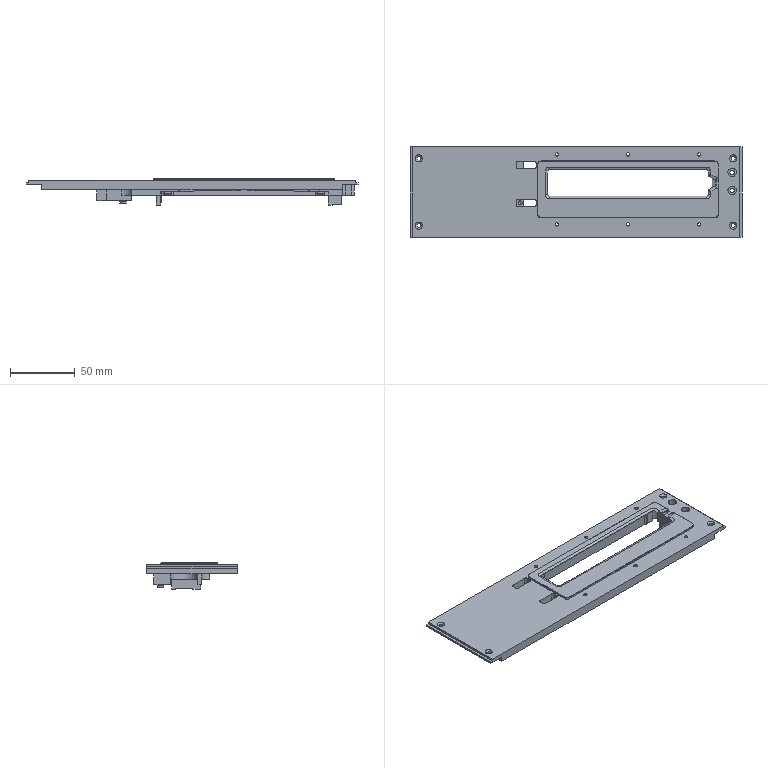NC program | NX | posted with a generic post | part box 256.6 x 70.3 x 20.422 mm
Lines 23 to 1070 of 15201:
(ADAPTIVE_MILLING , TOOL : D10)
N44 T10 M6
N46 G54
N48 G17 G0 G90 X-140.009 Y0.038 S9500 M3
N50 G43 Z30. H10
N52 Z-17.422
N54 G94 G1 Z-20.422 F1000.
N56 X-139.228 Y-0.241 F3000.
N58 X-138.44 Y-0.497
N60 G3 X-137.362 Y0.038 R1.017
N62 X-136.601 Y3.102 R8.28
N64 X-136.319 Y12.969 R111.643
N66 G1 X-136.314 Y15.219
N68 X-136.311 Y19.094
N70 X-136.31 Y32.719
N72 Y36.094
N74 X-136.305 Y36.344
N76 X-136.296 Y36.469
N78 G2 X-133.53 Y40.732 R5.992
N80 X-127.787 Y42.697 R13.242
N82 X-118.803 Y43.116 R74.905
N84 G1 X-117.428 Y43.124
N86 X-115.678 Y43.13
N88 X-113.178 Y43.135
N90 X-108.678 Y43.137
N92 X-67.178 Y43.138
N94 X129.322
N96 G2 X133.647 Y40.731 R5.631
N98 X135.753 Y35.309 R12.113
N100 X136.254 Y27.082 R56.828
N102 G1 X136.263 Y26.082
N104 X136.272 Y24.832
N106 X136.279 Y23.207
N108 X136.284 Y21.082
N110 X136.287 Y17.457
N112 X136.288 Y6.457
N114 Y-36.168
N116 X136.287 Y-36.293
N118 X136.281 Y-36.417
N120 X136.271 Y-36.542
N122 G2 X133.571 Y-40.712 R5.953
N124 X128.205 Y-42.64 R12.812
N126 X120.225 Y-43.103 R59.248
N128 G1 X119.225 Y-43.113
N130 X117.975 Y-43.122
N132 X116.35 Y-43.129
N134 X114.1 Y-43.134
N136 X110.35 Y-43.137
N138 X98.35 Y-43.138
N140 X1.1
N142 X0.475 Y-43.141
N144 X-1.275 Y-43.144
N146 X-2.9
N148 X-3.4 Y-43.143
N150 X-4.025 Y-43.145
N152 X-5.4 Y-43.146
N154 X-6.275 Y-43.145
N156 X-7.025 Y-43.147
N158 X-7.9
N160 X-8.525 Y-43.146
N162 X-9.65 Y-43.149
N164 X-10.525 Y-43.147
N166 X-11.65 Y-43.149
N168 X-12.65 Y-43.147
N170 X-13.525 Y-43.149
N172 X-15.025 Y-43.147
N174 X-15.775 Y-43.148
N176 X-16.775 Y-43.147
N178 X-17.4 Y-43.148
N180 X-18.275 Y-43.15
N182 X-19.15 Y-43.148
N184 X-20.4 Y-43.15
N186 X-21.65 Y-43.147
N188 X-22.275 Y-43.149
N190 X-23.775 Y-43.147
N192 X-24.525 Y-43.146
N194 X-25.275 Y-43.148
N196 X-26.15 Y-43.147
N198 X-26.525
N200 X-27.775 Y-43.15
N202 X-28.525 Y-43.148
N204 X-29.775 Y-43.15
N206 X-31.025 Y-43.147
N208 X-31.65 Y-43.148
N210 X-33.025 Y-43.147
N212 X-33.774 Y-43.146
N214 X-34.399 Y-43.147
N216 X-35.774
N218 X-36.524 Y-43.146
N220 X-37.399 Y-43.148
N222 X-38.524 Y-43.147
N224 X-39.399 Y-43.149
N226 X-40.399 Y-43.147
N228 X-40.899 Y-43.146
N230 X-41.649 Y-43.148
N232 X-42.649 Y-43.147
N234 X-43.274 Y-43.148
N236 X-44.149 Y-43.15
N238 X-45.024 Y-43.148
N240 X-46.149 Y-43.15
N242 X-46.899 Y-43.149
N244 X-48.149 Y-43.15
N246 X-49.524 Y-43.147
N248 X-50.899 Y-43.15
N250 X-52.024 Y-43.148
N252 X-52.774 Y-43.149
N254 X-54.024 Y-43.148
N256 X-54.899 Y-43.149
N258 X-56.024 Y-43.148
N260 X-57.149 Y-43.15
N262 X-58.149 Y-43.148
N264 X-59.274 Y-43.15
N266 X-60.024 Y-43.149
N268 X-60.899
N270 X-61.274 Y-43.15
N272 X-62.649 Y-43.147
N274 X-64.024 Y-43.15
N276 X-65.149 Y-43.148
N278 X-65.899 Y-43.149
N280 X-67.149 Y-43.148
N282 X-68.024 Y-43.149
N284 X-69.024 Y-43.148
N286 X-70.274 Y-43.15
N288 X-71.024 Y-43.149
N290 X-71.899 Y-43.15
N292 X-72.524 Y-43.151
N294 X-73.774 Y-43.148
N296 X-74.399 Y-43.149
N298 X-75.899 Y-43.148
N300 X-76.524 Y-43.147
N302 X-77.399 Y-43.149
N304 X-78.524 Y-43.147
N306 X-79.274 Y-43.149
N308 X-80.524 Y-43.147
N310 X-81.899 Y-43.15
N312 X-83.274 Y-43.147
N314 X-84.274 Y-43.149
N316 X-85.274 Y-43.147
N318 X-86.524 Y-43.15
N320 X-87.774 Y-43.147
N322 X-88.899 Y-43.15
N324 X-89.524 Y-43.149
N326 X-90.899 Y-43.15
N328 X-91.649 Y-43.151
N330 X-92.399 Y-43.149
N332 X-93.274 Y-43.15
N334 X-93.774 Y-43.151
N336 X-94.649 Y-43.149
N338 X-95.899 Y-43.151
N340 X-97.149 Y-43.148
N342 X-97.774 Y-43.149
N344 X-99.274 Y-43.148
N346 X-99.899 Y-43.146
N348 X-100.774 Y-43.149
N350 X-101.899 Y-43.147
N352 X-102.774 Y-43.149
N354 X-104.149 Y-43.147
N356 X-105.024 Y-43.149
N358 X-106.149 Y-43.147
N360 X-107.024 Y-43.149
N362 X-108.399 Y-43.147
N364 X-109.274 Y-43.149
N366 X-110.399 Y-43.147
N368 X-111.274 Y-43.149
N370 X-112.649 Y-43.147
N372 X-113.524 Y-43.149
N374 X-114.649 Y-43.147
N376 X-115.399 Y-43.149
N378 X-116.649 Y-43.147
N380 X-117.899 Y-43.15
N382 X-118.649 Y-43.148
N384 X-119.524 Y-43.149
N386 X-120.024 Y-43.15
N388 X-120.899 Y-43.148
N390 X-122.274 Y-43.151
N392 X-123.024 Y-43.149
N394 X-123.899 Y-43.15
N396 X-124.399 Y-43.151
N398 X-125.399 Y-43.148
N400 X-126.149 Y-43.15
N402 X-127.149 Y-43.148
N404 X-127.524
N406 X-128.524 Y-43.15
N408 X-129.274 Y-43.148
N410 X-129.399 Y-43.146
N412 X-129.524 Y-43.142
N414 X-129.649 Y-43.134
N416 X-129.773 Y-43.122
N418 G2 X-133.906 Y-40.362 R5.979
N420 X-135.817 Y-34.86 R13.054
N422 X-136.263 Y-26.128 R68.977
N424 G1 X-136.272 Y-24.753
N426 X-136.279 Y-23.253
N428 X-136.284 Y-21.003
N430 X-136.287 Y-17.253
N432 X-136.288 Y-5.128
N434 Y-3.753
N436 G2 X-135.756 Y1.844 R63.19
N438 G3 X-135.334 Y14.457 R138.248
N440 G1 X-135.328 Y16.582
N442 X-135.324 Y19.582
N444 X-135.321 Y25.082
N446 Y32.957
N448 X-135.318 Y33.207
N450 X-135.315 Y33.332
N452 G2 X-131.585 Y39.496 R7.69
N454 X-125.11 Y41.636 R15.73
N456 X-115.127 Y42.102 R84.01
N458 G1 X-113.877 Y42.11
N460 X-112.252 Y42.117
N462 X-109.877 Y42.122
N464 X-106.127 Y42.126
N466 X-96.502 Y42.127
N468 X4.498
N470 X5.248 Y42.131
N472 X6.373 Y42.133
N474 X7.248 Y42.132
N476 X7.998 Y42.135
N478 X9.123
N480 X9.498 Y42.134
N482 X10.373 Y42.137
N484 X11.373 Y42.135
N486 X11.998 Y42.134
N488 X12.623 Y42.136
N490 X14.123
N492 X15.123 Y42.134
N494 X15.873 Y42.137
N496 X16.873 Y42.136
N498 X17.248 Y42.135
N500 X18.498 Y42.138
N502 X19.498 Y42.136
N504 X20.248 Y42.138
N506 X21.373 Y42.137
N508 X21.748 Y42.136
N510 X22.873 Y42.139
N512 X24.248 Y42.136
N514 X25.498 Y42.139
N516 X26.123 Y42.138
N518 X27.623 Y42.139
N520 X28.498 Y42.14
N522 X29.373 Y42.138
N524 X30.623 Y42.14
N526 X31.873 Y42.137
N528 X32.623 Y42.139
N530 X33.623 Y42.137
N532 X33.998
N534 X35.248 Y42.139
N536 X36.248 Y42.137
N538 X36.998 Y42.138
N540 X38.123 Y42.137
N542 X38.748 Y42.136
N544 X39.748 Y42.138
N546 X40.623 Y42.137
N548 X41.873 Y42.139
N550 X42.998 Y42.137
N552 X44.373 Y42.14
N554 X45.623 Y42.137
N556 X46.998 Y42.14
N558 X48.248 Y42.137
N560 X48.873 Y42.138
N562 X50.373 Y42.137
N564 X51.248 Y42.135
N566 X52.248 Y42.138
N568 X52.998 Y42.137
N570 X54.123 Y42.138
N572 X54.498 Y42.139
N574 X55.748 Y42.136
N576 X56.748 Y42.139
N578 X57.498 Y42.138
N580 X58.623 Y42.139
N582 X59.248 Y42.14
N584 X60.248 Y42.138
N586 X61.123 Y42.139
N588 X62.373 Y42.137
N590 X63.498 Y42.139
N592 X64.873 Y42.136
N594 X65.498 Y42.137
N596 X66.998
N598 X67.998 Y42.135
N600 X68.873 Y42.138
N602 X69.498 Y42.137
N604 X70.373 Y42.135
N606 X71.123 Y42.137
N608 X72.248 Y42.136
N610 X72.873 Y42.137
N612 X73.373 Y42.138
N614 X74.123 Y42.137
N616 X74.748 Y42.136
N618 X75.873 Y42.139
N620 X76.873 Y42.137
N622 X78.248 Y42.14
N624 X79.498 Y42.137
N626 X80.873 Y42.14
N628 X82.123 Y42.137
N630 X82.748 Y42.138
N632 X84.248 Y42.137
N634 X85.123 Y42.135
N636 X85.998 Y42.138
N638 X86.623 Y42.137
N640 X87.373 Y42.135
N642 X88.373 Y42.138
N644 X89.123 Y42.137
N646 X90.248 Y42.138
N648 X90.873 Y42.14
N650 X91.873 Y42.137
N652 X92.623 Y42.139
N654 X93.748 Y42.137
N656 X94.123
N658 X95.373 Y42.139
N660 X96.373 Y42.137
N662 X97.123 Y42.138
N664 X98.248 Y42.137
N666 X98.873 Y42.136
N668 X99.748 Y42.138
N670 X100.373 Y42.137
N672 X101.123 Y42.136
N674 X101.998 Y42.138
N676 X102.623 Y42.137
N678 X103.373 Y42.136
N680 X104.373 Y42.138
N682 X105.123 Y42.137
N684 X106.248 Y42.139
N686 X106.748 Y42.14
N688 X107.998 Y42.137
N690 X108.748 Y42.138
N692 X109.748 Y42.137
N694 X110.123 Y42.136
N696 X111.373 Y42.139
N698 X112.373 Y42.137
N700 X113.123 Y42.138
N702 X114.248 Y42.137
N704 X114.623
N706 X115.873 Y42.139
N708 X116.873 Y42.137
N710 X118.123 Y42.14
N712 G2 X126.996 Y42.1 R280.962
N714 X132.731 Y38.306 R7.752
N716 X134.81 Y31.809 R16.037
N718 X135.251 Y22.2 R84.671
N720 G1 X135.26 Y20.825
N722 X135.267 Y19.2
N724 X135.273 Y16.95
N726 X135.276 Y13.325
N728 X135.277 Y3.825
N730 X135.278 Y-33.05
N732 G2 X131.69 Y-39.417 R7.605
N734 X125.239 Y-41.62 R15.293
N736 X115.882 Y-42.096 R77.581
N738 G1 X114.632 Y-42.106
N740 X113.007 Y-42.115
N742 X111.007 Y-42.12
N744 X108.007 Y-42.125
N746 X102.132 Y-42.127
N748 X4.132
N750 X3.257 Y-42.131
N752 X1.757 Y-42.135
N754 X0.257 Y-42.136
N756 X-0.368
N758 X-1.243 Y-42.14
N760 X-2.368
N762 X-3.118 Y-42.142
N764 X-4.118
N766 X-5.118 Y-42.145
N768 X-6.118 Y-42.144
N770 X-6.868 Y-42.146
N772 X-7.993 Y-42.145
N774 X-8.368
N776 X-9.118 Y-42.147
N778 X-10.118 Y-42.146
N780 X-10.743 Y-42.147
N782 X-11.368 Y-42.149
N784 X-12.118 Y-42.147
N786 X-13.243 Y-42.148
N788 X-13.743 Y-42.149
N790 X-14.618 Y-42.147
N792 X-15.618 Y-42.149
N794 X-16.493 Y-42.148
N796 X-17.743 Y-42.15
N798 X-19.118 Y-42.147
N800 X-19.868 Y-42.149
N802 X-20.993 Y-42.147
N804 X-21.618 Y-42.146
N806 X-22.368 Y-42.147
N808 X-23.618 Y-42.146
N810 X-24.118 Y-42.145
N812 X-24.993 Y-42.148
N814 X-25.993 Y-42.147
N816 X-26.618
N818 X-27.243 Y-42.149
N820 X-28.243 Y-42.147
N822 X-29.243 Y-42.149
N824 X-30.743 Y-42.145
N826 X-31.618 Y-42.147
N828 X-32.618 Y-42.146
N830 X-33.493 Y-42.144
N832 X-34.493 Y-42.147
N834 X-35.743 Y-42.145
N836 X-36.868 Y-42.148
N838 X-38.118 Y-42.145
N840 X-39.243 Y-42.148
N842 X-40.368 Y-42.146
N844 X-41.618 Y-42.149
N846 X-42.493 Y-42.148
N848 X-43.743 Y-42.15
N850 X-44.743 Y-42.148
N852 X-45.743 Y-42.15
N854 X-46.618 Y-42.148
N856 X-47.493 Y-42.149
N858 X-47.993 Y-42.15
N860 X-49.243 Y-42.148
N862 X-50.243 Y-42.15
N864 X-51.493 Y-42.147
N866 X-52.493 Y-42.149
N868 X-53.243 Y-42.148
N870 X-54.368 Y-42.149
N872 X-54.743 Y-42.15
N874 X-55.743 Y-42.148
N876 X-56.618 Y-42.15
N878 X-57.743 Y-42.148
N880 X-58.618 Y-42.15
N882 X-59.493 Y-42.148
N884 X-59.868
N886 X-61.243 Y-42.15
N888 X-62.243 Y-42.148
N890 X-63.118 Y-42.149
N892 X-63.993 Y-42.148
N894 X-64.368 Y-42.147
N896 X-65.368 Y-42.149
N898 X-66.243 Y-42.148
N900 X-67.118 Y-42.149
N902 X-67.618 Y-42.15
N904 X-68.868 Y-42.148
N906 X-69.868 Y-42.15
N908 X-71.118 Y-42.148
N910 X-72.243 Y-42.15
N912 X-73.618 Y-42.147
N914 X-74.868 Y-42.149
N916 X-75.743 Y-42.147
N918 X-76.993 Y-42.149
N920 X-77.743 Y-42.148
N922 X-78.868 Y-42.149
N924 X-79.368 Y-42.15
N926 X-80.618 Y-42.147
N928 X-81.743 Y-42.15
N930 X-82.743 Y-42.147
N932 X-83.743 Y-42.15
N934 X-84.743 Y-42.148
N936 X-86.118 Y-42.15
N938 X-87.493 Y-42.147
N940 X-88.368 Y-42.15
N942 X-89.118 Y-42.149
N944 X-89.743 Y-42.148
N946 X-90.743 Y-42.15
N948 X-91.743 Y-42.149
N950 X-92.618 Y-42.15
N952 X-92.993 Y-42.151
N954 X-94.243 Y-42.148
N956 X-95.118 Y-42.15
N958 X-95.868 Y-42.148
N960 X-96.493 Y-42.147
N962 X-97.868 Y-42.15
N964 X-98.993 Y-42.147
N966 X-99.868 Y-42.149
N968 X-100.743 Y-42.147
N970 X-101.243 Y-42.146
N972 X-102.243 Y-42.148
N974 X-103.368 Y-42.146
N976 X-104.493 Y-42.149
N978 X-105.493 Y-42.146
N980 X-106.493 Y-42.148
N982 X-107.743 Y-42.146
N984 X-108.493 Y-42.148
N986 X-109.618 Y-42.147
N988 X-110.118 Y-42.146
N990 X-111.118 Y-42.148
N992 X-111.993 Y-42.147
N994 X-113.243 Y-42.149
N996 X-114.243 Y-42.147
N998 X-114.993 Y-42.149
N1000 X-116.243 Y-42.148
N1002 X-116.618 Y-42.147
N1004 X-117.368 Y-42.149
N1006 G2 X-126.867 Y-42.12 R653.766
N1008 X-132.789 Y-38.202 R7.786
N1010 X-134.807 Y-31.812 R16.325
N1012 X-135.25 Y-22.328 R83.36
N1014 X-135.231 Y-4.204 R701.54
N1016 G3 X-134.546 Y5.271 R671.484
N1018 X-134.335 Y21.643 R413.405
N1020 G2 X-134.291 Y31.392 R372.601
N1022 X-133.486 Y34.523 R9.347
N1024 X-133.248 Y36.547 R27.401
N1026 X-130.811 Y39.637 R5.458
N1028 X-128.265 Y40.3 R6.048
N1030 X-113.92 Y41.084 R119.555
N1032 G1 X-112.546 Y41.095
N1034 X-111.171 Y41.102
N1036 X-109.046 Y41.108
N1038 X-106.046 Y41.113
N1040 X-100.796 Y41.116
N1042 X-68.671
N1044 X1.454
N1046 X2.329 Y41.121
N1048 X3.454 Y41.124
N1050 X4.329
N1052 X5.079 Y41.127
N1054 X6.204 Y41.129
N1056 X7.204
N1058 X7.954 Y41.132
N1060 X8.954
N1062 X9.329
N1064 X10.579 Y41.135
N1066 X11.329 Y41.134
N1068 X12.579 Y41.136
N1070 X12.954 Y41.137
N1072 X13.704 Y41.136
N1074 X14.829 Y41.137
N1076 X15.579 Y41.139
N1078 X16.454 Y41.137
N1080 X17.329 Y41.138
N1082 X17.829 Y41.139
N1084 X19.079 Y41.136
N1086 X20.079 Y41.138
N1088 X20.704 Y41.137
N1090 X21.454 Y41.135
N1092 X22.704 Y41.139
N1094 X23.454 Y41.138
N1096 X24.704 Y41.139
N1098 X25.579 Y41.141
N1100 X26.829 Y41.138
N1102 X28.079 Y41.141
N1104 X28.954 Y41.139
N1106 X30.204
N1108 X30.829 Y41.14
N1110 X31.704 Y41.138
N1112 X32.954 Y41.14
N1114 X33.704 Y41.138
N1116 X34.829 Y41.139
N1118 X35.204 Y41.14
N1120 X36.079 Y41.138
N1122 X37.079 Y41.139
N1124 X37.704
N1126 X38.579 Y41.136
N1128 X39.454 Y41.138
N1130 X40.704 Y41.136
N1132 X41.829 Y41.139
N1134 X43.079 Y41.136
N1136 X44.204 Y41.139
N1138 X44.829 Y41.138
N1140 X45.329 Y41.137
N1142 X46.329 Y41.139
N1144 X48.204 Y41.134
N1146 X49.454 Y41.138
N1148 X50.704 Y41.135
N1150 X51.829 Y41.138
N1152 X52.954 Y41.136
N1154 X54.204 Y41.139
N1156 X55.329 Y41.136
N1158 X56.204 Y41.138
N1160 X57.329
N1162 X57.954 Y41.137
N1164 X58.704 Y41.138
N1166 X59.829 Y41.137
N1168 X60.204 Y41.136
N1170 X61.079 Y41.138
N1172 X62.204 Y41.136
N1174 X63.329 Y41.139
N1176 X64.954 Y41.134
N1178 X66.079 Y41.137
N1180 X67.329 Y41.135
N1182 X68.329 Y41.137
N1184 X69.704 Y41.134
N1186 X70.454 Y41.136
N1188 X71.704 Y41.135
N1190 X72.204
N1192 X73.329 Y41.138
N1194 X74.204 Y41.136
N1196 X75.454 Y41.138
N1198 X76.579 Y41.136
N1200 X77.704 Y41.139
N1202 X78.829 Y41.136
N1204 X79.204
N1206 X79.954 Y41.137
N1208 X81.204 Y41.136
N1210 X82.079 Y41.134
N1212 X83.454 Y41.138
N1214 X84.579 Y41.135
N1216 X85.704 Y41.138
N1218 X86.829 Y41.136
N1220 X88.079 Y41.139
N1222 X89.204 Y41.137
N1224 X90.204 Y41.139
N1226 X91.579 Y41.136
N1228 X92.829 Y41.139
N1230 X93.954 Y41.137
N1232 X94.954 Y41.139
N1234 X96.079 Y41.136
N1236 X97.329 Y41.139
N1238 X98.204 Y41.137
N1240 X99.204 Y41.138
N1242 X99.954
N1244 X100.704 Y41.136
N1246 X101.704 Y41.137
N1248 X102.954 Y41.136
N1250 X104.204 Y41.139
N1252 X105.204 Y41.137
N1254 X106.204 Y41.138
N1256 X107.329 Y41.136
N1258 X108.329 Y41.138
N1260 X109.329 Y41.137
N1262 X109.954
N1264 X110.704 Y41.139
N1266 X112.079 Y41.136
N1268 X113.329 Y41.139
N1270 X114.454 Y41.137
N1272 X115.204 Y41.138
N1274 X116.454
N1276 X117.079 Y41.137
N1278 X118.079 Y41.139
N1280 X118.954 Y41.137
N1282 X119.954 Y41.139
N1284 G2 X125.076 Y41.051 R57.765
N1286 X127.716 Y40.316 R11.925
N1288 X129.697 Y40.098 R13.373
N1290 X132.787 Y37.661 R5.458
N1292 X133.445 Y35.184 R5.984
N1294 X134.237 Y20.465 R121.517
N1296 G1 X134.247 Y19.09
N1298 X134.254 Y17.34
N1300 X134.26 Y15.09
N1302 X134.264 Y11.715
N1304 X134.266 Y4.965
N1306 X134.267 Y-30.41
N1308 G2 X133.486 Y-34.427 R9.489
N1310 X133.248 Y-36.547 R22.386
N1312 X130.811 Y-39.637 R5.458
N1314 X128.334 Y-40.295 R5.984
N1316 X112.49 Y-41.095 R131.095
N1318 G1 X110.74 Y-41.103
N1320 X108.49 Y-41.109
N1322 X105.24 Y-41.114
N1324 X99.24 Y-41.116
N1326 X7.115
N1328 X6.24 Y-41.121
N1330 X5.115 Y-41.124
N1332 X2.49 Y-41.125
N1334 X1.74 Y-41.129
N1336 X0.115 Y-41.134
N1338 X-1.385 Y-41.135
N1340 X-2.01 Y-41.137
N1342 X-2.385 Y-41.139
N1344 X-3.385
N1346 X-3.76
N1348 X-4.76 Y-41.143
N1350 X-5.76 Y-41.142
N1352 X-6.76 Y-41.145
N1354 X-7.76 Y-41.144
N1356 X-8.635 Y-41.146
N1358 X-9.385
N1360 X-9.885 Y-41.145
N1362 X-11.135 Y-41.148
N1364 X-12.26 Y-41.146
N1366 X-13.135 Y-41.148
N1368 X-14.26 Y-41.147
N1370 X-15.135 Y-41.149
N1372 X-15.885 Y-41.148
N1374 X-16.51 Y-41.146
N1376 X-17.385 Y-41.148
N1378 X-18.385 Y-41.146
N1380 X-18.885 Y-41.145
N1382 X-19.635 Y-41.147
N1384 X-20.885 Y-41.145
N1386 X-21.26
N1388 X-22.135 Y-41.146
N1390 X-23.01
N1392 X-23.51 Y-41.145
N1394 X-24.76 Y-41.148
N1396 X-25.76 Y-41.146
N1398 X-26.51 Y-41.148
N1400 X-27.635 Y-41.147
N1402 X-28.26 Y-41.146
N1404 X-29.385 Y-41.148
N1406 X-30.51 Y-41.145
N1408 X-31.51 Y-41.147
N1410 X-32.26 Y-41.145
N1412 X-32.76 Y-41.144
N1414 X-33.885 Y-41.147
N1416 X-34.51 Y-41.146
N1418 X-35.135 Y-41.144
N1420 X-36.385 Y-41.147
N1422 X-37.51 Y-41.145
N1424 X-38.885 Y-41.149
N1426 X-40.01 Y-41.146
N1428 X-40.76 Y-41.148
N1430 X-42.01
N1432 X-42.635 Y-41.147
N1434 X-43.26 Y-41.148
N1436 X-44.51
N1438 X-46.385 Y-41.144
N1440 X-47.635 Y-41.148
N1442 X-48.885 Y-41.146
N1444 X-49.885 Y-41.148
N1446 X-50.76 Y-41.147
N1448 X-51.51 Y-41.148
N1450 X-52.01 Y-41.149
N1452 X-53.26 Y-41.147
N1454 X-54.135 Y-41.149
N1456 X-55.385 Y-41.147
N1458 X-56.385 Y-41.15
N1460 X-57.135 Y-41.148
N1462 X-58.385 Y-41.149
N1464 X-58.885 Y-41.15
N1466 X-60.01 Y-41.148
N1468 X-60.76 Y-41.149
N1470 X-61.635 Y-41.148
N1472 X-62.01
N1474 X-63.135 Y-41.15
N1476 X-64.01 Y-41.148
N1478 X-65.26 Y-41.15
N1480 X-66.01 Y-41.149
N1482 X-67.135 Y-41.15
N1484 X-67.635 Y-41.151
N1486 X-68.385 Y-41.149
N1488 X-69.51 Y-41.15
N1490 X-69.885 Y-41.151
N1492 X-71.01 Y-41.148
N1494 X-72.135 Y-41.15
N1496 X-73.135 Y-41.148
N1498 X-74.51 Y-41.151
N1500 X-75.26 Y-41.149
N1502 X-76.385 Y-41.15
N1504 X-76.76 Y-41.151
N1506 X-77.635 Y-41.149
N1508 X-78.635 Y-41.15
N1510 X-79.01
N1512 X-79.885 Y-41.149
N1514 X-80.76 Y-41.15
N1516 X-81.135
N1518 X-82.135 Y-41.148
N1520 X-83.26 Y-41.15
N1522 X-84.76 Y-41.147
N1524 X-85.885 Y-41.15
N1526 X-86.76 Y-41.148
N1528 X-87.635 Y-41.149
N1530 X-88.135 Y-41.15
N1532 X-89.385 Y-41.148
N1534 X-90.385 Y-41.15
N1536 X-91.635 Y-41.148
N1538 X-92.76 Y-41.15
N1540 X-93.635 Y-41.148
N1542 X-94.76 Y-41.149
N1544 X-95.385 Y-41.15
N1546 X-96.385 Y-41.148
N1548 X-97.51 Y-41.15
N1550 X-98.385 Y-41.148
N1552 X-99.635 Y-41.149
N1554 X-100.76 Y-41.146
N1556 X-102.01 Y-41.149
N1558 X-103.01 Y-41.147
N1560 X-103.76 Y-41.148
N1562 X-104.885 Y-41.147
N1564 X-105.385 Y-41.146
N1566 X-106.135 Y-41.147
N1568 X-107.26 Y-41.146
N1570 X-107.635
N1572 X-108.51 Y-41.147
N1574 X-109.76 Y-41.146
N1576 X-110.51 Y-41.147
N1578 X-111.635
N1580 X-112.01 Y-41.146
N1582 G2 X-124.634 Y-41.105 R449.34
N1584 X-127.646 Y-40.332 R9.422
N1586 X-129.697 Y-40.098 R20.63
N1588 X-132.787 Y-37.661 R5.458
N1590 X-133.445 Y-35.184 R5.984
N1592 X-134.242 Y-19.715 R126.881
N1594 X-134.213 Y-5.216 R537.427
N1596 G3 X-133.531 Y6.389 R774.372
N1598 G1 X-133.506 Y7.138
N1600 X-133.48 Y8.013
N1602 X-133.457 Y8.888
N1604 X-133.45 Y9.176
N1606 Y34.801
N1608 G2 X-132.718 Y37.78 R5.923
N1610 X-129.564 Y40.134 R5.458
N1612 G1 X-128.265 Y40.3
N1614 X127.86
N1616 G2 X130.93 Y39.568 R5.969
N1618 X133.284 Y36.414 R5.458
N1620 G1 X133.445 Y35.184
N1622 X133.45 Y35.115
N1624 Y-34.635
N1626 G2 X132.718 Y-37.78 R6.018
N1628 X129.564 Y-40.134 R5.458
N1630 G1 X128.334 Y-40.295
N1632 X128.265 Y-40.3
N1634 X-127.86
N1636 G2 X-130.93 Y-39.568 R5.969
N1638 X-133.284 Y-36.414 R5.458
N1640 G1 X-133.445 Y-35.184
N1642 X-133.45 Y-35.115
N1644 Y9.26
N1646 G3 X-134.303 Y10.258 R1.016
N1648 G1 X-135.881 Y10.505
N1650 Z-17.422
N1652 G0 Z30.
N1654 X-125.86 Y-42.8
N1656 Z0.04
N1658 G1 Z-2.96 F1000.
N1660 X-126.107 Y-41.094 F3000.
N1662 G3 X-126.975 Y-40.237 R1.017
N1664 G2 X-129.13 Y-39.568 R5.238
N1666 X-131.63 Y-35.806 R5.552
N1668 X-132.293 Y-28.472 R39.509
N1670 X-132.359 Y-13.473 R778.304
N1672 G1 Y32.277
N1674 X-132.357 Y32.402
N1676 X-132.35 Y32.527
N1678 X-132.339 Y32.651
N1680 G2 X-131.692 Y34.662 R6.357
N1682 G1 X-131.664 Y34.784
N1684 X-131.65 Y34.884
N1686 Y35.115
N1688 X-131.645 Y35.184
N1690 X-131.484 Y36.414
N1692 X-131.448 Y36.547
N1694 G2 X-129.011 Y39.637 R5.458
N1696 X-127.02 Y40.232 R5.27
N1698 G3 X-126.625 Y42.073 R1.001
N1700 X-127.256 Y42.258 Z-2.927 R1.72
N1702 G1 X-128.572 Y42.495 Z-2.86
N1704 X-129.38 Y42.647
N1706 X-130.193 Y42.774
N1708 G3 X-130.917 Y42.482 R1.026
N1710 G1 X-131.744 Y41.657
N1712 X-132.558 Y40.821
N1714 G3 X-134.132 Y38.041 R7.74
N1716 X-135.244 Y32.57 R22.257
N1718 X-135.418 Y27.584 R74.022
N1720 G1 X-135.381 Y-34.164
N1722 G3 X-135.161 Y-34.788 R1.04
N1724 G1 X-133.969 Y-36.279
N1726 X-133.563 Y-36.794 Z-2.893
N1728 X-133.137 Y-37.294 Z-2.925
N1730 G3 X-132.512 Y-37.544 Z-2.96 R1.039
N1732 X-131.484 Y-36.414 R1.004
N1734 G1 X-131.645 Y-35.184
N1736 X-131.65 Y-35.115
N1738 Y34.885
N1740 G3 X-132.677 Y35.895 R1.014
N1742 G1 X-134.074 Y35.872
N1744 Z0.04
N1746 G0 Z30.
N1748 X125.819 Y42.8
N1750 Z0.04
N1752 G1 Z-2.96 F1000.
N1754 X126.075 Y41.093 F3000.
N1756 G3 X126.942 Y40.242 R1.017
N1758 G2 X129.13 Y39.568 R5.274
N1760 X131.629 Y35.806 R5.54
N1762 X132.293 Y28.472 R39.245
N1764 X132.359 Y13.348 R783.285
N1766 G1 Y-32.152
N1768 X132.358 Y-32.277
N1770 X132.356 Y-32.402
N1772 X132.351 Y-32.527
N1774 X132.341 Y-32.652
N1776 G2 X131.705 Y-34.665 R5.662
N1778 G1 X131.672 Y-34.785
N1780 X131.65 Y-34.919
N1782 Y-35.115
N1784 X131.645 Y-35.184
N1786 X131.484 Y-36.414
N1788 X131.448 Y-36.547
N1790 G2 X129.011 Y-39.637 R5.458
N1792 X127.02 Y-40.232 R5.27
N1794 G3 X126.625 Y-42.073 R1.001
N1796 X127.256 Y-42.258 Z-2.927 R1.72
N1798 G1 X128.572 Y-42.495 Z-2.86
N1800 X129.38 Y-42.647
N1802 X130.193 Y-42.774
N1804 G3 X130.917 Y-42.482 R1.026
N1806 G1 X131.744 Y-41.657
N1808 X132.558 Y-40.821
N1810 G3 X134.132 Y-38.041 R7.74
N1812 G1 X134.506 Y-36.851
N1814 X134.836 Y-35.647
N1816 G3 X135.289 Y-32.263 R19.614
N1818 G1 X135.35 Y-30.861
N1820 X135.376 Y-29.459
N1822 X135.381 Y34.164
N1824 G3 X135.161 Y34.789 R1.039
N1826 G1 X134.043 Y36.187
N1828 X133.605 Y36.737 Z-2.895
N1830 X133.155 Y37.278 Z-2.93
N1832 G3 X132.629 Y37.532 Z-2.96 R1.049
N1834 X131.484 Y36.414 R1.003
N1836 G1 X131.645 Y35.184
N1838 X131.65 Y35.115
N1840 Y-35.01
N1842 G3 X132.654 Y-36.02 R1.014
N1844 G1 X134.053 Y-36.029
N1846 Z0.04
N1848 G0 Z30.
N1850 X-134.106 Y-1.313
N1852 Z1.751
N1854 G1 Z-1.249 F1000.
N1856 X-133.059 Y-0.797 F3000.
N1858 X-132.022 Y-0.261
N1860 X-131.858 Y-0.113
N1862 X-131.725 Y0.063
N1864 G3 X-130.942 Y2.86 R6.974
N1866 X-130.625 Y11.475 R84.168
N1868 G1 X-130.619 Y13.1
N1870 X-130.614 Y15.475
N1872 X-130.611 Y19.6
N1874 X-130.61 Y31.975
N1876 X-130.607 Y32.35
N1878 X-130.602 Y32.474
N1880 G2 X-128.02 Y36.709 R5.802
N1882 X-122.555 Y38.713 R12.557
N1884 X-113.7 Y39.185 R65.122
N1886 G1 X-112.575 Y39.193
N1888 X-111.075 Y39.201
N1890 X-108.95 Y39.207
N1892 X-105.575 Y39.21
N1894 X-96.825 Y39.213
N1896 X-27.075 Y39.221
N1898 X-26.325 Y39.225
N1900 X-25.2 Y39.227
N1902 X-24.325
N1904 X-23.575 Y39.229
N1906 X-22.45
N1908 X-22.075
N1910 X-21.2 Y39.231
N1912 X-20.2 Y39.23
N1914 X-19.7 Y39.229
N1916 X-19.075 Y39.231
N1918 X-17.7
N1920 X-16.95 Y39.23
N1922 X-15.95 Y39.233
N1924 X-14.7 Y39.231
N1926 X-13.95 Y39.233
N1928 X-12.95 Y39.232
N1930 X-12.575 Y39.231
N1932 X-11.325 Y39.234
N1934 X-10.45 Y39.233
N1936 X-9.2 Y39.235
N1938 X-7.825 Y39.232
N1940 X-7.2 Y39.234
N1942 X-5.7 Y39.233
N1944 X-4.7 Y39.232
N1946 X-3.825 Y39.234
N1948 X-3.2 Y39.233
N1950 X-2.45 Y39.232
N1952 X-1.575 Y39.234
N1954 X-0.95
N1956 X-0.2 Y39.232
N1958 X0.675 Y39.235
N1960 X1.3 Y39.234
N1962 X2.05 Y39.233
N1964 X2.925 Y39.235
N1966 X3.55 Y39.234
N1968 X4.3 Y39.233
N1970 X5.175 Y39.235
N1972 X5.8
N1974 X6.55 Y39.233
N1976 X7.425 Y39.235
N1978 X8.05
N1980 X8.8 Y39.233
N1982 X9.8 Y39.236
N1984 X10.55 Y39.235
N1986 X11.675 Y39.237
N1988 X12.175 Y39.238
N1990 X13.425 Y39.235
N1992 X14.175 Y39.237
N1994 X15.175 Y39.236
N1996 X15.675 Y39.235
N1998 X16.55 Y39.237
N2000 X17.55 Y39.236
N2002 X18.549 Y39.238
N2004 X19.674 Y39.236
N2006 X20.924 Y39.239
N2008 X21.674 Y39.237
N2010 X22.674 Y39.238
N2012 X23.174 Y39.239
N2014 X24.049 Y39.238
N2016 X25.174 Y39.239
N2018 X26.424 Y39.237
N2020 X27.424 Y39.239
N2022 X28.799 Y39.236
N2024 X30.049 Y39.24
N2026 X30.674 Y39.238
N2028 X32.174 Y39.239
N2030 X33.049 Y39.241
N2032 X33.924 Y39.239
N2034 X34.549 Y39.24
N2036 X35.299 Y39.241
N2038 X36.299 Y39.239
N2040 X37.049 Y39.24
N2042 X38.174 Y39.239
N2044 X38.674 Y39.238
N2046 X39.924 Y39.241
N2048 X40.674 Y39.239
N2050 X41.674 Y39.241
N2052 X42.049
N2054 X43.299 Y39.239
N2056 X44.299 Y39.241
N2058 X45.049 Y39.24
N2060 X46.174 Y39.241
N2062 X46.549 Y39.242
N2064 X47.799 Y39.239
N2066 X48.799 Y39.241
N2068 X50.049 Y39.239
N2070 X50.799 Y39.241
N2072 X51.674 Y39.24
N2074 X52.174 Y39.239
N2076 X53.174 Y39.242
N2078 X54.049 Y39.24
N2080 X55.424 Y39.243
N2082 X56.424 Y39.241
N2084 X57.674 Y39.243
N2086 X58.424 Y39.242
N2088 X59.299 Y39.243
N2090 X59.799 Y39.244
N2092 X60.799 Y39.241
N2094 X61.674 Y39.243
N2096 X63.174 Y39.24
N2098 X64.049 Y39.243
N2100 X65.299 Y39.241
N2102 X66.549 Y39.244
N2104 X67.424 Y39.242
N2106 X68.674 Y39.244
N2108 X69.424 Y39.243
N2110 X70.549 Y39.245
N2112 X71.174 Y39.244
N2114 X72.174 Y39.242
N2116 X72.924 Y39.243
N2118 X73.924
N2120 X74.424 Y39.242
N2122 X75.174 Y39.243
N2124 X76.299 Y39.242
N2126 X76.924 Y39.243
N2128 X77.799 Y39.245
N2130 X78.674 Y39.243
N2132 X79.924 Y39.246